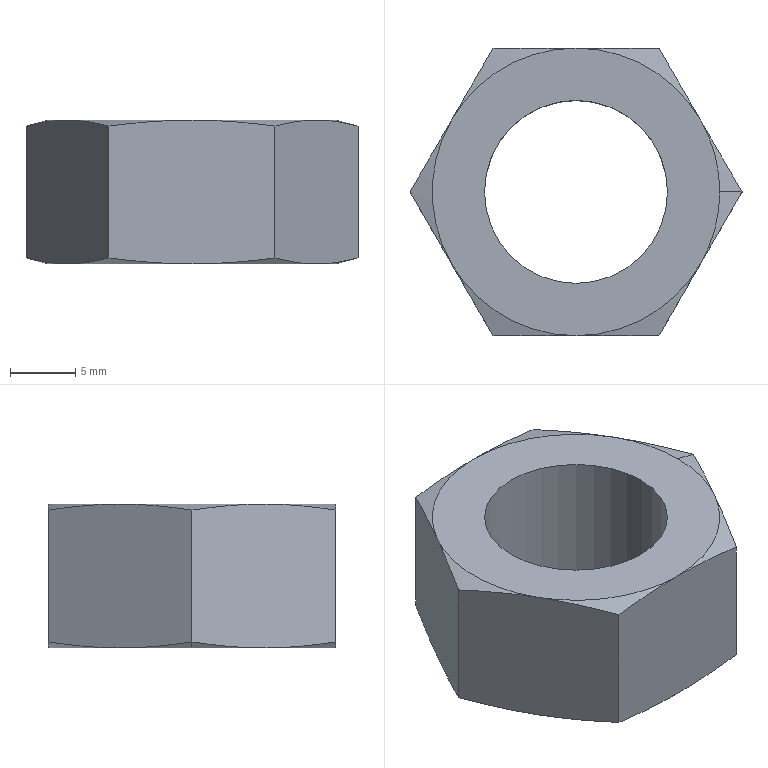Part | SolidWorks | features Cut 2, Chamfer 1, Extrusion 1 | 1 solid | 24 faces | box 25.4 x 21.997 x 11 mm | volume 2905 mm3 | cone 14 | plane 8 | cylinder 2 | commonest cylinder face diameters 14 x2
STEP:
#1=CARTESIAN_POINT('',(10.999,0.,11.));
#2=VERTEX_POINT('',#1);
#3=CARTESIAN_POINT('',(9.525,5.499,11.));
#4=VERTEX_POINT('',#3);
#5=CARTESIAN_POINT('',(0.,0.,11.));
#6=DIRECTION('',(0.,0.,1.));
#7=DIRECTION('',(1.,0.,0.));
#8=AXIS2_PLACEMENT_3D('',#5,#6,#7);
#9=CIRCLE('',#8,10.999);
#10=EDGE_CURVE('',#2,#4,#9,.T.);
#11=ORIENTED_EDGE('',*,*,#10,.F.);
#12=CARTESIAN_POINT('',(12.7,0.,10.544));
#13=VERTEX_POINT('',#12);
#14=CARTESIAN_POINT('',(10.999,0.,11.));
#15=DIRECTION('',(0.9659,0.,-0.2588));
#16=VECTOR('',#15,1000.);
#17=LINE('',#14,#16);
#18=EDGE_CURVE('',#2,#13,#17,.T.);
#19=ORIENTED_EDGE('',*,*,#18,.T.);
#20=CARTESIAN_POINT('',(12.7,0.,10.544));
#21=CARTESIAN_POINT('',(12.171,0.9165,10.686));
#22=CARTESIAN_POINT('',(11.642,1.833,10.801));
#23=CARTESIAN_POINT('',(10.583,3.666,10.958));
#24=CARTESIAN_POINT('',(10.054,4.583,11.));
#25=CARTESIAN_POINT('',(9.525,5.499,11.));
#26=B_SPLINE_CURVE_WITH_KNOTS('',3,(#20,#21,#22,#23,#24,#25),.UNSPECIFIED.,.F.,.F.,(4,2,4),(0.000000231,0.003175,0.00635),.UNSPECIFIED.);
#27=EDGE_CURVE('',#13,#4,#26,.T.);
#28=ORIENTED_EDGE('',*,*,#27,.T.);
#29=EDGE_LOOP('',(#11,#19,#28));
#30=FACE_OUTER_BOUND('',#29,.T.);
#31=CARTESIAN_POINT('',(0.,0.,11.));
#32=DIRECTION('',(0.,0.,-1.));
#33=DIRECTION('',(1.,0.,0.));
#34=AXIS2_PLACEMENT_3D('',#31,#32,#33);
#35=CONICAL_SURFACE('',#34,10.999,1.309);
#36=ADVANCED_FACE('',(#30),#35,.T.);
#37=CARTESIAN_POINT('',(-10.999,0.,0.));
#38=VERTEX_POINT('',#37);
#39=CARTESIAN_POINT('',(-9.525,5.499,0.));
#40=VERTEX_POINT('',#39);
#41=CARTESIAN_POINT('',(0.,0.,0.));
#42=DIRECTION('',(0.,0.,-1.));
#43=DIRECTION('',(-1.,0.,0.));
#44=AXIS2_PLACEMENT_3D('',#41,#42,#43);
#45=CIRCLE('',#44,10.999);
#46=EDGE_CURVE('',#38,#40,#45,.T.);
#47=ORIENTED_EDGE('',*,*,#46,.F.);
#48=CARTESIAN_POINT('',(-12.7,0.,0.4559));
#49=VERTEX_POINT('',#48);
#50=CARTESIAN_POINT('',(-10.999,0.,0.));
#51=DIRECTION('',(-0.9659,0.,0.2588));
#52=VECTOR('',#51,1000.);
#53=LINE('',#50,#52);
#54=EDGE_CURVE('',#38,#49,#53,.T.);
#55=ORIENTED_EDGE('',*,*,#54,.T.);
#56=CARTESIAN_POINT('',(-12.7,0.,0.4559));
#57=CARTESIAN_POINT('',(-12.171,0.9165,0.3141));
#58=CARTESIAN_POINT('',(-11.642,1.833,0.199));
#59=CARTESIAN_POINT('',(-10.583,3.666,0.04169));
#60=CARTESIAN_POINT('',(-10.054,4.583,0.));
#61=CARTESIAN_POINT('',(-9.525,5.499,0.));
#62=B_SPLINE_CURVE_WITH_KNOTS('',3,(#56,#57,#58,#59,#60,#61),.UNSPECIFIED.,.F.,.F.,(4,2,4),(0.000000231,0.003175,0.00635),.UNSPECIFIED.);
#63=EDGE_CURVE('',#49,#40,#62,.T.);
#64=ORIENTED_EDGE('',*,*,#63,.T.);
#65=EDGE_LOOP('',(#47,#55,#64));
#66=FACE_OUTER_BOUND('',#65,.T.);
#67=CARTESIAN_POINT('',(0.,0.,0.));
#68=DIRECTION('',(0.,0.,1.));
#69=DIRECTION('',(-1.,0.,0.));
#70=AXIS2_PLACEMENT_3D('',#67,#68,#69);
#71=CONICAL_SURFACE('',#70,10.999,1.309);
#72=ADVANCED_FACE('',(#66),#71,.T.);
#73=CARTESIAN_POINT('',(-7.,0.,11.));
#74=VERTEX_POINT('',#73);
#75=CARTESIAN_POINT('',(7.,0.,11.));
#76=VERTEX_POINT('',#75);
#77=CARTESIAN_POINT('',(0.,0.,11.));
#78=DIRECTION('',(0.,0.,1.));
#79=DIRECTION('',(1.,0.,0.));
#80=AXIS2_PLACEMENT_3D('',#77,#78,#79);
#81=CIRCLE('',#80,7.);
#82=EDGE_CURVE('',#74,#76,#81,.T.);
#83=ORIENTED_EDGE('',*,*,#82,.T.);
#84=CARTESIAN_POINT('',(7.,0.,0.));
#85=VERTEX_POINT('',#84);
#86=CARTESIAN_POINT('',(7.,0.,11.));
#87=DIRECTION('',(0.,0.,-1.));
#88=VECTOR('',#87,1000.);
#89=LINE('',#86,#88);
#90=EDGE_CURVE('',#76,#85,#89,.T.);
#91=ORIENTED_EDGE('',*,*,#90,.T.);
#92=CARTESIAN_POINT('',(-7.,0.,0.));
#93=VERTEX_POINT('',#92);
#94=CARTESIAN_POINT('',(0.,0.,0.));
#95=DIRECTION('',(0.,0.,1.));
#96=DIRECTION('',(1.,0.,0.));
#97=AXIS2_PLACEMENT_3D('',#94,#95,#96);
#98=CIRCLE('',#97,7.);
#99=EDGE_CURVE('',#93,#85,#98,.T.);
#100=ORIENTED_EDGE('',*,*,#99,.F.);
#101=CARTESIAN_POINT('',(-7.,0.,11.));
#102=DIRECTION('',(0.,0.,-1.));
#103=VECTOR('',#102,1000.);
#104=LINE('',#101,#103);
#105=EDGE_CURVE('',#74,#93,#104,.T.);
#106=ORIENTED_EDGE('',*,*,#105,.F.);
#107=EDGE_LOOP('',(#83,#91,#100,#106));
#108=FACE_OUTER_BOUND('',#107,.T.);
#109=CARTESIAN_POINT('',(0.,0.,11.));
#110=DIRECTION('',(0.,0.,-1.));
#111=DIRECTION('',(-1.,0.,0.));
#112=AXIS2_PLACEMENT_3D('',#109,#110,#111);
#113=CYLINDRICAL_SURFACE('',#112,7.);
#114=ADVANCED_FACE('',(#108),#113,.F.);
#115=ORIENTED_EDGE('',*,*,#27,.F.);
#116=CARTESIAN_POINT('',(12.7,0.,0.4559));
#117=VERTEX_POINT('',#116);
#118=CARTESIAN_POINT('',(12.7,0.,11.));
#119=DIRECTION('',(0.,0.,-1.));
#120=VECTOR('',#119,1000.);
#121=LINE('',#118,#120);
#122=EDGE_CURVE('',#13,#117,#121,.T.);
#123=ORIENTED_EDGE('',*,*,#122,.T.);
#124=CARTESIAN_POINT('',(9.525,5.499,0.));
#125=VERTEX_POINT('',#124);
#126=CARTESIAN_POINT('',(9.525,5.499,0.));
#127=CARTESIAN_POINT('',(10.054,4.583,0.));
#128=CARTESIAN_POINT('',(10.583,3.666,0.04169));
#129=CARTESIAN_POINT('',(11.642,1.833,0.199));
#130=CARTESIAN_POINT('',(12.171,0.9165,0.3141));
#131=CARTESIAN_POINT('',(12.7,0.,0.4559));
#132=B_SPLINE_CURVE_WITH_KNOTS('',3,(#126,#127,#128,#129,#130,#131),.UNSPECIFIED.,.F.,.F.,(4,2,4),(0.00635,0.009525,0.0127),.UNSPECIFIED.);
#133=EDGE_CURVE('',#125,#117,#132,.T.);
#134=ORIENTED_EDGE('',*,*,#133,.F.);
#135=CARTESIAN_POINT('',(6.35,10.999,0.4559));
#136=VERTEX_POINT('',#135);
#137=CARTESIAN_POINT('',(6.35,10.999,0.4559));
#138=CARTESIAN_POINT('',(6.879,10.082,0.3141));
#139=CARTESIAN_POINT('',(7.408,9.165,0.199));
#140=CARTESIAN_POINT('',(8.467,7.332,0.04169));
#141=CARTESIAN_POINT('',(8.996,6.416,0.));
#142=CARTESIAN_POINT('',(9.525,5.499,0.));
#143=B_SPLINE_CURVE_WITH_KNOTS('',3,(#137,#138,#139,#140,#141,#142),.UNSPECIFIED.,.F.,.F.,(4,2,4),(0.000000231,0.003175,0.00635),.UNSPECIFIED.);
#144=EDGE_CURVE('',#136,#125,#143,.T.);
#145=ORIENTED_EDGE('',*,*,#144,.F.);
#146=CARTESIAN_POINT('',(6.35,10.999,10.544));
#147=VERTEX_POINT('',#146);
#148=CARTESIAN_POINT('',(6.35,10.999,11.));
#149=DIRECTION('',(0.,0.,-1.));
#150=VECTOR('',#149,1000.);
#151=LINE('',#148,#150);
#152=EDGE_CURVE('',#147,#136,#151,.T.);
#153=ORIENTED_EDGE('',*,*,#152,.F.);
#154=CARTESIAN_POINT('',(9.525,5.499,11.));
#155=CARTESIAN_POINT('',(8.996,6.416,11.));
#156=CARTESIAN_POINT('',(8.467,7.332,10.958));
#157=CARTESIAN_POINT('',(7.408,9.165,10.801));
#158=CARTESIAN_POINT('',(6.879,10.082,10.686));
#159=CARTESIAN_POINT('',(6.35,10.999,10.544));
#160=B_SPLINE_CURVE_WITH_KNOTS('',3,(#154,#155,#156,#157,#158,#159),.UNSPECIFIED.,.F.,.F.,(4,2,4),(0.00635,0.009525,0.0127),.UNSPECIFIED.);
#161=EDGE_CURVE('',#4,#147,#160,.T.);
#162=ORIENTED_EDGE('',*,*,#161,.F.);
#163=EDGE_LOOP('',(#115,#123,#134,#145,#153,#162));
#164=FACE_OUTER_BOUND('',#163,.T.);
#165=CARTESIAN_POINT('',(12.7,0.,11.));
#166=DIRECTION('',(-0.866,-0.5,0.));
#167=DIRECTION('',(0.5,-0.866,0.));
#168=AXIS2_PLACEMENT_3D('',#165,#166,#167);
#169=PLANE('',#168);
#170=ADVANCED_FACE('',(#164),#169,.F.);
#171=CARTESIAN_POINT('',(0.,10.999,11.));
#172=VERTEX_POINT('',#171);
#173=CARTESIAN_POINT('',(6.35,10.999,10.544));
#174=CARTESIAN_POINT('',(5.293,10.999,10.686));
#175=CARTESIAN_POINT('',(4.236,10.999,10.801));
#176=CARTESIAN_POINT('',(2.12,10.999,10.958));
#177=CARTESIAN_POINT('',(1.06,10.999,11.));
#178=CARTESIAN_POINT('',(0.,10.999,11.));
#179=B_SPLINE_CURVE_WITH_KNOTS('',3,(#173,#174,#175,#176,#177,#178),.UNSPECIFIED.,.F.,.F.,(4,2,4),(0.03237,0.03557,0.03876),.UNSPECIFIED.);
#180=EDGE_CURVE('',#147,#172,#179,.T.);
#181=ORIENTED_EDGE('',*,*,#180,.F.);
#182=ORIENTED_EDGE('',*,*,#152,.T.);
#183=CARTESIAN_POINT('',(0.,10.999,0.));
#184=VERTEX_POINT('',#183);
#185=CARTESIAN_POINT('',(0.,10.999,0.));
#186=CARTESIAN_POINT('',(1.06,10.999,0.));
#187=CARTESIAN_POINT('',(2.12,10.999,0.04184));
#188=CARTESIAN_POINT('',(4.236,10.999,0.1993));
#189=CARTESIAN_POINT('',(5.293,10.999,0.3144));
#190=CARTESIAN_POINT('',(6.35,10.999,0.4559));
#191=B_SPLINE_CURVE_WITH_KNOTS('',3,(#185,#186,#187,#188,#189,#190),.UNSPECIFIED.,.F.,.F.,(4,2,4),(0.01717,0.02038,0.02358),.UNSPECIFIED.);
#192=EDGE_CURVE('',#184,#136,#191,.T.);
#193=ORIENTED_EDGE('',*,*,#192,.F.);
#194=CARTESIAN_POINT('',(-6.35,10.999,0.4559));
#195=VERTEX_POINT('',#194);
#196=CARTESIAN_POINT('',(-6.35,10.999,0.4559));
#197=CARTESIAN_POINT('',(-5.295,10.999,0.3145));
#198=CARTESIAN_POINT('',(-4.233,10.999,0.1989));
#199=CARTESIAN_POINT('',(-2.115,10.999,0.04158));
#200=CARTESIAN_POINT('',(-1.057,10.999,0.));
#201=CARTESIAN_POINT('',(0.,10.999,0.));
#202=B_SPLINE_CURVE_WITH_KNOTS('',3,(#196,#197,#198,#199,#200,#201),.UNSPECIFIED.,.F.,.F.,(4,2,4),(0.01079,0.01398,0.01717),.UNSPECIFIED.);
#203=EDGE_CURVE('',#195,#184,#202,.T.);
#204=ORIENTED_EDGE('',*,*,#203,.F.);
#205=CARTESIAN_POINT('',(-6.35,10.999,10.544));
#206=VERTEX_POINT('',#205);
#207=CARTESIAN_POINT('',(-6.35,10.999,11.));
#208=DIRECTION('',(0.,0.,-1.));
#209=VECTOR('',#208,1000.);
#210=LINE('',#207,#209);
#211=EDGE_CURVE('',#206,#195,#210,.T.);
#212=ORIENTED_EDGE('',*,*,#211,.F.);
#213=CARTESIAN_POINT('',(0.,10.999,11.));
#214=CARTESIAN_POINT('',(-1.057,10.999,11.));
#215=CARTESIAN_POINT('',(-2.115,10.999,10.958));
#216=CARTESIAN_POINT('',(-4.233,10.999,10.801));
#217=CARTESIAN_POINT('',(-5.295,10.999,10.685));
#218=CARTESIAN_POINT('',(-6.35,10.999,10.544));
#219=B_SPLINE_CURVE_WITH_KNOTS('',3,(#213,#214,#215,#216,#217,#218),.UNSPECIFIED.,.F.,.F.,(4,2,4),(0.03876,0.04194,0.04513),.UNSPECIFIED.);
#220=EDGE_CURVE('',#172,#206,#219,.T.);
#221=ORIENTED_EDGE('',*,*,#220,.F.);
#222=EDGE_LOOP('',(#181,#182,#193,#204,#212,#221));
#223=FACE_OUTER_BOUND('',#222,.T.);
#224=CARTESIAN_POINT('',(6.35,10.999,11.));
#225=DIRECTION('',(0.,-1.,0.));
#226=DIRECTION('',(1.,0.,0.));
#227=AXIS2_PLACEMENT_3D('',#224,#225,#226);
#228=PLANE('',#227);
#229=ADVANCED_FACE('',(#223),#228,.F.);
#230=CARTESIAN_POINT('',(-9.525,5.499,11.));
#231=VERTEX_POINT('',#230);
#232=CARTESIAN_POINT('',(-6.35,10.999,10.544));
#233=CARTESIAN_POINT('',(-6.879,10.082,10.686));
#234=CARTESIAN_POINT('',(-7.408,9.165,10.801));
#235=CARTESIAN_POINT('',(-8.467,7.332,10.958));
#236=CARTESIAN_POINT('',(-8.996,6.416,11.));
#237=CARTESIAN_POINT('',(-9.525,5.499,11.));
#238=B_SPLINE_CURVE_WITH_KNOTS('',3,(#232,#233,#234,#235,#236,#237),.UNSPECIFIED.,.F.,.F.,(4,2,4),(0.000000231,0.003175,0.00635),.UNSPECIFIED.);
#239=EDGE_CURVE('',#206,#231,#238,.T.);
#240=ORIENTED_EDGE('',*,*,#239,.F.);
#241=ORIENTED_EDGE('',*,*,#211,.T.);
#242=CARTESIAN_POINT('',(-9.525,5.499,0.));
#243=CARTESIAN_POINT('',(-8.996,6.416,0.));
#244=CARTESIAN_POINT('',(-8.467,7.332,0.04169));
#245=CARTESIAN_POINT('',(-7.408,9.165,0.199));
#246=CARTESIAN_POINT('',(-6.879,10.082,0.3141));
#247=CARTESIAN_POINT('',(-6.35,10.999,0.4559));
#248=B_SPLINE_CURVE_WITH_KNOTS('',3,(#242,#243,#244,#245,#246,#247),.UNSPECIFIED.,.F.,.F.,(4,2,4),(0.00635,0.009525,0.0127),.UNSPECIFIED.);
#249=EDGE_CURVE('',#40,#195,#248,.T.);
#250=ORIENTED_EDGE('',*,*,#249,.F.);
#251=ORIENTED_EDGE('',*,*,#63,.F.);
#252=CARTESIAN_POINT('',(-12.7,0.,10.544));
#253=VERTEX_POINT('',#252);
#254=CARTESIAN_POINT('',(-12.7,0.,11.));
#255=DIRECTION('',(0.,0.,-1.));
#256=VECTOR('',#255,1000.);
#257=LINE('',#254,#256);
#258=EDGE_CURVE('',#253,#49,#257,.T.);
#259=ORIENTED_EDGE('',*,*,#258,.F.);
#260=CARTESIAN_POINT('',(-9.525,5.499,11.));
#261=CARTESIAN_POINT('',(-10.054,4.583,11.));
#262=CARTESIAN_POINT('',(-10.583,3.666,10.958));
#263=CARTESIAN_POINT('',(-11.642,1.833,10.801));
#264=CARTESIAN_POINT('',(-12.171,0.9165,10.686));
#265=CARTESIAN_POINT('',(-12.7,0.,10.544));
#266=B_SPLINE_CURVE_WITH_KNOTS('',3,(#260,#261,#262,#263,#264,#265),.UNSPECIFIED.,.F.,.F.,(4,2,4),(0.00635,0.009525,0.0127),.UNSPECIFIED.);
#267=EDGE_CURVE('',#231,#253,#266,.T.);
#268=ORIENTED_EDGE('',*,*,#267,.F.);
#269=EDGE_LOOP('',(#240,#241,#250,#251,#259,#268));
#270=FACE_OUTER_BOUND('',#269,.T.);
#271=CARTESIAN_POINT('',(-6.35,10.999,11.));
#272=DIRECTION('',(0.866,-0.5,0.));
#273=DIRECTION('',(0.5,0.866,0.));
#274=AXIS2_PLACEMENT_3D('',#271,#272,#273);
#275=PLANE('',#274);
#276=ADVANCED_FACE('',(#270),#275,.F.);
#277=CARTESIAN_POINT('',(-9.525,-5.499,11.));
#278=VERTEX_POINT('',#277);
#279=CARTESIAN_POINT('',(-12.7,0.,10.544));
#280=CARTESIAN_POINT('',(-12.171,-0.9165,10.686));
#281=CARTESIAN_POINT('',(-11.642,-1.833,10.801));
#282=CARTESIAN_POINT('',(-10.583,-3.666,10.958));
#283=CARTESIAN_POINT('',(-10.054,-4.583,11.));
#284=CARTESIAN_POINT('',(-9.525,-5.499,11.));
#285=B_SPLINE_CURVE_WITH_KNOTS('',3,(#279,#280,#281,#282,#283,#284),.UNSPECIFIED.,.F.,.F.,(4,2,4),(0.000000231,0.003175,0.00635),.UNSPECIFIED.);
#286=EDGE_CURVE('',#253,#278,#285,.T.);
#287=ORIENTED_EDGE('',*,*,#286,.F.);
#288=ORIENTED_EDGE('',*,*,#258,.T.);
#289=CARTESIAN_POINT('',(-9.525,-5.499,0.));
#290=VERTEX_POINT('',#289);
#291=CARTESIAN_POINT('',(-9.525,-5.499,0.));
#292=CARTESIAN_POINT('',(-10.054,-4.583,0.));
#293=CARTESIAN_POINT('',(-10.583,-3.666,0.04169));
#294=CARTESIAN_POINT('',(-11.642,-1.833,0.199));
#295=CARTESIAN_POINT('',(-12.171,-0.9165,0.3141));
#296=CARTESIAN_POINT('',(-12.7,0.,0.4559));
#297=B_SPLINE_CURVE_WITH_KNOTS('',3,(#291,#292,#293,#294,#295,#296),.UNSPECIFIED.,.F.,.F.,(4,2,4),(0.00635,0.009525,0.0127),.UNSPECIFIED.);
#298=EDGE_CURVE('',#290,#49,#297,.T.);
#299=ORIENTED_EDGE('',*,*,#298,.F.);
#300=CARTESIAN_POINT('',(-6.35,-10.999,0.4559));
#301=VERTEX_POINT('',#300);
#302=CARTESIAN_POINT('',(-6.35,-10.999,0.4559));
#303=CARTESIAN_POINT('',(-6.879,-10.082,0.3141));
#304=CARTESIAN_POINT('',(-7.408,-9.165,0.199));
#305=CARTESIAN_POINT('',(-8.467,-7.332,0.04169));
#306=CARTESIAN_POINT('',(-8.996,-6.416,0.));
#307=CARTESIAN_POINT('',(-9.525,-5.499,0.));
#308=B_SPLINE_CURVE_WITH_KNOTS('',3,(#302,#303,#304,#305,#306,#307),.UNSPECIFIED.,.F.,.F.,(4,2,4),(0.000000231,0.003175,0.00635),.UNSPECIFIED.);
#309=EDGE_CURVE('',#301,#290,#308,.T.);
#310=ORIENTED_EDGE('',*,*,#309,.F.);
#311=CARTESIAN_POINT('',(-6.35,-10.999,10.544));
#312=VERTEX_POINT('',#311);
#313=CARTESIAN_POINT('',(-6.35,-10.999,11.));
#314=DIRECTION('',(0.,0.,-1.));
#315=VECTOR('',#314,1000.);
#316=LINE('',#313,#315);
#317=EDGE_CURVE('',#312,#301,#316,.T.);
#318=ORIENTED_EDGE('',*,*,#317,.F.);
#319=CARTESIAN_POINT('',(-9.525,-5.499,11.));
#320=CARTESIAN_POINT('',(-8.996,-6.416,11.));
#321=CARTESIAN_POINT('',(-8.467,-7.332,10.958));
#322=CARTESIAN_POINT('',(-7.408,-9.165,10.801));
#323=CARTESIAN_POINT('',(-6.879,-10.082,10.686));
#324=CARTESIAN_POINT('',(-6.35,-10.999,10.544));
#325=B_SPLINE_CURVE_WITH_KNOTS('',3,(#319,#320,#321,#322,#323,#324),.UNSPECIFIED.,.F.,.F.,(4,2,4),(0.00635,0.009525,0.0127),.UNSPECIFIED.);
#326=EDGE_CURVE('',#278,#312,#325,.T.);
#327=ORIENTED_EDGE('',*,*,#326,.F.);
#328=EDGE_LOOP('',(#287,#288,#299,#310,#318,#327));
#329=FACE_OUTER_BOUND('',#328,.T.);
#330=CARTESIAN_POINT('',(-12.7,0.,11.));
#331=DIRECTION('',(0.866,0.5,0.));
#332=DIRECTION('',(-0.5,0.866,0.));
#333=AXIS2_PLACEMENT_3D('',#330,#331,#332);
#334=PLANE('',#333);
#335=ADVANCED_FACE('',(#329),#334,.F.);
#336=CARTESIAN_POINT('',(0.,-10.999,11.));
#337=VERTEX_POINT('',#336);
#338=CARTESIAN_POINT('',(-6.35,-10.999,10.544));
#339=CARTESIAN_POINT('',(-5.295,-10.999,10.685));
#340=CARTESIAN_POINT('',(-4.233,-10.999,10.801));
#341=CARTESIAN_POINT('',(-2.115,-10.999,10.958));
#342=CARTESIAN_POINT('',(-1.057,-10.999,11.));
#343=CARTESIAN_POINT('',(0.,-10.999,11.));
#344=B_SPLINE_CURVE_WITH_KNOTS('',3,(#338,#339,#340,#341,#342,#343),.UNSPECIFIED.,.F.,.F.,(4,2,4),(0.01079,0.01398,0.01717),.UNSPECIFIED.);
#345=EDGE_CURVE('',#312,#337,#344,.T.);
#346=ORIENTED_EDGE('',*,*,#345,.F.);
#347=ORIENTED_EDGE('',*,*,#317,.T.);
#348=CARTESIAN_POINT('',(0.,-10.999,0.));
#349=VERTEX_POINT('',#348);
#350=CARTESIAN_POINT('',(0.,-10.999,0.));
#351=CARTESIAN_POINT('',(-1.057,-10.999,0.));
#352=CARTESIAN_POINT('',(-2.115,-10.999,0.04158));
#353=CARTESIAN_POINT('',(-4.233,-10.999,0.1989));
#354=CARTESIAN_POINT('',(-5.295,-10.999,0.3145));
#355=CARTESIAN_POINT('',(-6.35,-10.999,0.4559));
#356=B_SPLINE_CURVE_WITH_KNOTS('',3,(#350,#351,#352,#353,#354,#355),.UNSPECIFIED.,.F.,.F.,(4,2,4),(0.03876,0.04194,0.04513),.UNSPECIFIED.);
#357=EDGE_CURVE('',#349,#301,#356,.T.);
#358=ORIENTED_EDGE('',*,*,#357,.F.);
#359=CARTESIAN_POINT('',(6.35,-10.999,0.4559));
#360=VERTEX_POINT('',#359);
#361=CARTESIAN_POINT('',(6.35,-10.999,0.4559));
#362=CARTESIAN_POINT('',(5.293,-10.999,0.3144));
#363=CARTESIAN_POINT('',(4.236,-10.999,0.1993));
#364=CARTESIAN_POINT('',(2.12,-10.999,0.04184));
#365=CARTESIAN_POINT('',(1.06,-10.999,0.));
#366=CARTESIAN_POINT('',(0.,-10.999,0.));
#367=B_SPLINE_CURVE_WITH_KNOTS('',3,(#361,#362,#363,#364,#365,#366),.UNSPECIFIED.,.F.,.F.,(4,2,4),(0.03237,0.03557,0.03876),.UNSPECIFIED.);
#368=EDGE_CURVE('',#360,#349,#367,.T.);
#369=ORIENTED_EDGE('',*,*,#368,.F.);
#370=CARTESIAN_POINT('',(6.35,-10.999,10.544));
#371=VERTEX_POINT('',#370);
#372=CARTESIAN_POINT('',(6.35,-10.999,11.));
#373=DIRECTION('',(0.,0.,-1.));
#374=VECTOR('',#373,1000.);
#375=LINE('',#372,#374);
#376=EDGE_CURVE('',#371,#360,#375,.T.);
#377=ORIENTED_EDGE('',*,*,#376,.F.);
#378=CARTESIAN_POINT('',(0.,-10.999,11.));
#379=CARTESIAN_POINT('',(1.06,-10.999,11.));
#380=CARTESIAN_POINT('',(2.12,-10.999,10.958));
#381=CARTESIAN_POINT('',(4.236,-10.999,10.801));
#382=CARTESIAN_POINT('',(5.293,-10.999,10.686));
#383=CARTESIAN_POINT('',(6.35,-10.999,10.544));
#384=B_SPLINE_CURVE_WITH_KNOTS('',3,(#378,#379,#380,#381,#382,#383),.UNSPECIFIED.,.F.,.F.,(4,2,4),(0.01717,0.02038,0.02358),.UNSPECIFIED.);
#385=EDGE_CURVE('',#337,#371,#384,.T.);
#386=ORIENTED_EDGE('',*,*,#385,.F.);
#387=EDGE_LOOP('',(#346,#347,#358,#369,#377,#386));
#388=FACE_OUTER_BOUND('',#387,.T.);
#389=CARTESIAN_POINT('',(-6.35,-10.999,11.));
#390=DIRECTION('',(0.,1.,0.));
#391=DIRECTION('',(-1.,0.,0.));
#392=AXIS2_PLACEMENT_3D('',#389,#390,#391);
#393=PLANE('',#392);
#394=ADVANCED_FACE('',(#388),#393,.F.);
#395=CARTESIAN_POINT('',(9.525,-5.499,11.));
#396=VERTEX_POINT('',#395);
#397=CARTESIAN_POINT('',(6.35,-10.999,10.544));
#398=CARTESIAN_POINT('',(6.879,-10.082,10.686));
#399=CARTESIAN_POINT('',(7.408,-9.165,10.801));
#400=CARTESIAN_POINT('',(8.467,-7.332,10.958));
#401=CARTESIAN_POINT('',(8.996,-6.416,11.));
#402=CARTESIAN_POINT('',(9.525,-5.499,11.));
#403=B_SPLINE_CURVE_WITH_KNOTS('',3,(#397,#398,#399,#400,#401,#402),.UNSPECIFIED.,.F.,.F.,(4,2,4),(0.000000231,0.003175,0.00635),.UNSPECIFIED.);
#404=EDGE_CURVE('',#371,#396,#403,.T.);
#405=ORIENTED_EDGE('',*,*,#404,.F.);
#406=ORIENTED_EDGE('',*,*,#376,.T.);
#407=CARTESIAN_POINT('',(9.525,-5.499,0.));
#408=VERTEX_POINT('',#407);
#409=CARTESIAN_POINT('',(9.525,-5.499,0.));
#410=CARTESIAN_POINT('',(8.996,-6.416,0.));
#411=CARTESIAN_POINT('',(8.467,-7.332,0.04169));
#412=CARTESIAN_POINT('',(7.408,-9.165,0.199));
#413=CARTESIAN_POINT('',(6.879,-10.082,0.3141));
#414=CARTESIAN_POINT('',(6.35,-10.999,0.4559));
#415=B_SPLINE_CURVE_WITH_KNOTS('',3,(#409,#410,#411,#412,#413,#414),.UNSPECIFIED.,.F.,.F.,(4,2,4),(0.00635,0.009525,0.0127),.UNSPECIFIED.);
#416=EDGE_CURVE('',#408,#360,#415,.T.);
#417=ORIENTED_EDGE('',*,*,#416,.F.);
#418=CARTESIAN_POINT('',(12.7,0.,0.4559));
#419=CARTESIAN_POINT('',(12.171,-0.9165,0.3141));
#420=CARTESIAN_POINT('',(11.642,-1.833,0.199));
#421=CARTESIAN_POINT('',(10.583,-3.666,0.04169));
#422=CARTESIAN_POINT('',(10.054,-4.583,0.));
#423=CARTESIAN_POINT('',(9.525,-5.499,0.));
#424=B_SPLINE_CURVE_WITH_KNOTS('',3,(#418,#419,#420,#421,#422,#423),.UNSPECIFIED.,.F.,.F.,(4,2,4),(0.000000231,0.003175,0.00635),.UNSPECIFIED.);
#425=EDGE_CURVE('',#117,#408,#424,.T.);
#426=ORIENTED_EDGE('',*,*,#425,.F.);
#427=ORIENTED_EDGE('',*,*,#122,.F.);
#428=CARTESIAN_POINT('',(9.525,-5.499,11.));
#429=CARTESIAN_POINT('',(10.054,-4.583,11.));
#430=CARTESIAN_POINT('',(10.583,-3.666,10.958));
#431=CARTESIAN_POINT('',(11.642,-1.833,10.801));
#432=CARTESIAN_POINT('',(12.171,-0.9165,10.686));
#433=CARTESIAN_POINT('',(12.7,0.,10.544));
#434=B_SPLINE_CURVE_WITH_KNOTS('',3,(#428,#429,#430,#431,#432,#433),.UNSPECIFIED.,.F.,.F.,(4,2,4),(0.00635,0.009525,0.0127),.UNSPECIFIED.);
#435=EDGE_CURVE('',#396,#13,#434,.T.);
#436=ORIENTED_EDGE('',*,*,#435,.F.);
#437=EDGE_LOOP('',(#405,#406,#417,#426,#427,#436));
#438=FACE_OUTER_BOUND('',#437,.T.);
#439=CARTESIAN_POINT('',(6.35,-10.999,11.));
#440=DIRECTION('',(-0.866,0.5,0.));
#441=DIRECTION('',(-0.5,-0.866,0.));
#442=AXIS2_PLACEMENT_3D('',#439,#440,#441);
#443=PLANE('',#442);
#444=ADVANCED_FACE('',(#438),#443,.F.);
#445=ORIENTED_EDGE('',*,*,#82,.F.);
#446=CARTESIAN_POINT('',(0.,0.,11.));
#447=DIRECTION('',(0.,0.,1.));
#448=DIRECTION('',(1.,0.,0.));
#449=AXIS2_PLACEMENT_3D('',#446,#447,#448);
#450=CIRCLE('',#449,7.);
#451=EDGE_CURVE('',#76,#74,#450,.T.);
#452=ORIENTED_EDGE('',*,*,#451,.F.);
#453=EDGE_LOOP('',(#445,#452));
#454=FACE_BOUND('',#453,.T.);
#455=CARTESIAN_POINT('',(0.,0.,11.));
#456=DIRECTION('',(0.,0.,1.));
#457=DIRECTION('',(1.,0.,0.));
#458=AXIS2_PLACEMENT_3D('',#455,#456,#457);
#459=CIRCLE('',#458,10.999);
#460=EDGE_CURVE('',#396,#2,#459,.T.);
#461=ORIENTED_EDGE('',*,*,#460,.T.);
#462=ORIENTED_EDGE('',*,*,#10,.T.);
#463=CARTESIAN_POINT('',(0.,0.,11.));
#464=DIRECTION('',(0.,0.,1.));
#465=DIRECTION('',(1.,0.,0.));
#466=AXIS2_PLACEMENT_3D('',#463,#464,#465);
#467=CIRCLE('',#466,10.999);
#468=EDGE_CURVE('',#4,#172,#467,.T.);
#469=ORIENTED_EDGE('',*,*,#468,.T.);
#470=CARTESIAN_POINT('',(0.,0.,11.));
#471=DIRECTION('',(0.,0.,1.));
#472=DIRECTION('',(1.,0.,0.));
#473=AXIS2_PLACEMENT_3D('',#470,#471,#472);
#474=CIRCLE('',#473,10.999);
#475=EDGE_CURVE('',#172,#231,#474,.T.);
#476=ORIENTED_EDGE('',*,*,#475,.T.);
#477=CARTESIAN_POINT('',(0.,0.,11.));
#478=DIRECTION('',(0.,0.,1.));
#479=DIRECTION('',(1.,0.,0.));
#480=AXIS2_PLACEMENT_3D('',#477,#478,#479);
#481=CIRCLE('',#480,10.999);
#482=EDGE_CURVE('',#231,#278,#481,.T.);
#483=ORIENTED_EDGE('',*,*,#482,.T.);
#484=CARTESIAN_POINT('',(0.,0.,11.));
#485=DIRECTION('',(0.,0.,1.));
#486=DIRECTION('',(1.,0.,0.));
#487=AXIS2_PLACEMENT_3D('',#484,#485,#486);
#488=CIRCLE('',#487,10.999);
#489=EDGE_CURVE('',#278,#337,#488,.T.);
#490=ORIENTED_EDGE('',*,*,#489,.T.);
#491=CARTESIAN_POINT('',(0.,0.,11.));
#492=DIRECTION('',(0.,0.,1.));
#493=DIRECTION('',(1.,0.,0.));
#494=AXIS2_PLACEMENT_3D('',#491,#492,#493);
#495=CIRCLE('',#494,10.999);
#496=EDGE_CURVE('',#337,#396,#495,.T.);
#497=ORIENTED_EDGE('',*,*,#496,.T.);
#498=EDGE_LOOP('',(#461,#462,#469,#476,#483,#490,#497));
#499=FACE_OUTER_BOUND('',#498,.T.);
#500=CARTESIAN_POINT('',(6.35,10.999,11.));
#501=DIRECTION('',(0.,0.,1.));
#502=DIRECTION('',(1.,0.,0.));
#503=AXIS2_PLACEMENT_3D('',#500,#501,#502);
#504=PLANE('',#503);
#505=ADVANCED_FACE('',(#454,#499),#504,.T.);
#506=ORIENTED_EDGE('',*,*,#99,.T.);
#507=CARTESIAN_POINT('',(0.,0.,0.));
#508=DIRECTION('',(0.,0.,1.));
#509=DIRECTION('',(1.,0.,0.));
#510=AXIS2_PLACEMENT_3D('',#507,#508,#509);
#511=CIRCLE('',#510,7.);
#512=EDGE_CURVE('',#85,#93,#511,.T.);
#513=ORIENTED_EDGE('',*,*,#512,.T.);
#514=EDGE_LOOP('',(#506,#513));
#515=FACE_BOUND('',#514,.T.);
#516=CARTESIAN_POINT('',(0.,0.,0.));
#517=DIRECTION('',(0.,0.,-1.));
#518=DIRECTION('',(-1.,0.,0.));
#519=AXIS2_PLACEMENT_3D('',#516,#517,#518);
#520=CIRCLE('',#519,10.999);
#521=EDGE_CURVE('',#184,#125,#520,.T.);
#522=ORIENTED_EDGE('',*,*,#521,.T.);
#523=CARTESIAN_POINT('',(0.,0.,0.));
#524=DIRECTION('',(0.,0.,-1.));
#525=DIRECTION('',(-1.,0.,0.));
#526=AXIS2_PLACEMENT_3D('',#523,#524,#525);
#527=CIRCLE('',#526,10.999);
#528=EDGE_CURVE('',#125,#408,#527,.T.);
#529=ORIENTED_EDGE('',*,*,#528,.T.);
#530=CARTESIAN_POINT('',(0.,0.,0.));
#531=DIRECTION('',(0.,0.,-1.));
#532=DIRECTION('',(-1.,0.,0.));
#533=AXIS2_PLACEMENT_3D('',#530,#531,#532);
#534=CIRCLE('',#533,10.999);
#535=EDGE_CURVE('',#408,#349,#534,.T.);
#536=ORIENTED_EDGE('',*,*,#535,.T.);
#537=CARTESIAN_POINT('',(0.,0.,0.));
#538=DIRECTION('',(0.,0.,-1.));
#539=DIRECTION('',(-1.,0.,0.));
#540=AXIS2_PLACEMENT_3D('',#537,#538,#539);
#541=CIRCLE('',#540,10.999);
#542=EDGE_CURVE('',#349,#290,#541,.T.);
#543=ORIENTED_EDGE('',*,*,#542,.T.);
#544=CARTESIAN_POINT('',(0.,0.,0.));
#545=DIRECTION('',(0.,0.,-1.));
#546=DIRECTION('',(-1.,0.,0.));
#547=AXIS2_PLACEMENT_3D('',#544,#545,#546);
#548=CIRCLE('',#547,10.999);
#549=EDGE_CURVE('',#290,#38,#548,.T.);
#550=ORIENTED_EDGE('',*,*,#549,.T.);
#551=ORIENTED_EDGE('',*,*,#46,.T.);
#552=CARTESIAN_POINT('',(0.,0.,0.));
#553=DIRECTION('',(0.,0.,-1.));
#554=DIRECTION('',(-1.,0.,0.));
#555=AXIS2_PLACEMENT_3D('',#552,#553,#554);
#556=CIRCLE('',#555,10.999);
#557=EDGE_CURVE('',#40,#184,#556,.T.);
#558=ORIENTED_EDGE('',*,*,#557,.T.);
#559=EDGE_LOOP('',(#522,#529,#536,#543,#550,#551,#558));
#560=FACE_OUTER_BOUND('',#559,.T.);
#561=CARTESIAN_POINT('',(6.35,10.999,0.));
#562=DIRECTION('',(0.,0.,1.));
#563=DIRECTION('',(1.,0.,0.));
#564=AXIS2_PLACEMENT_3D('',#561,#562,#563);
#565=PLANE('',#564);
#566=ADVANCED_FACE('',(#515,#560),#565,.F.);
#567=ORIENTED_EDGE('',*,*,#90,.F.);
#568=ORIENTED_EDGE('',*,*,#451,.T.);
#569=ORIENTED_EDGE('',*,*,#105,.T.);
#570=ORIENTED_EDGE('',*,*,#512,.F.);
#571=EDGE_LOOP('',(#567,#568,#569,#570));
#572=FACE_OUTER_BOUND('',#571,.T.);
#573=CARTESIAN_POINT('',(0.,0.,11.));
#574=DIRECTION('',(0.,0.,-1.));
#575=DIRECTION('',(-1.,0.,0.));
#576=AXIS2_PLACEMENT_3D('',#573,#574,#575);
#577=CYLINDRICAL_SURFACE('',#576,7.);
#578=ADVANCED_FACE('',(#572),#577,.F.);
#579=ORIENTED_EDGE('',*,*,#368,.T.);
#580=ORIENTED_EDGE('',*,*,#535,.F.);
#581=ORIENTED_EDGE('',*,*,#416,.T.);
#582=EDGE_LOOP('',(#579,#580,#581));
#583=FACE_OUTER_BOUND('',#582,.T.);
#584=CARTESIAN_POINT('',(0.,0.,0.));
#585=DIRECTION('',(0.,0.,1.));
#586=DIRECTION('',(-1.,0.,0.));
#587=AXIS2_PLACEMENT_3D('',#584,#585,#586);
#588=CONICAL_SURFACE('',#587,10.999,1.309);
#589=ADVANCED_FACE('',(#583),#588,.T.);
#590=ORIENTED_EDGE('',*,*,#133,.T.);
#591=ORIENTED_EDGE('',*,*,#425,.T.);
#592=ORIENTED_EDGE('',*,*,#528,.F.);
#593=EDGE_LOOP('',(#590,#591,#592));
#594=FACE_OUTER_BOUND('',#593,.T.);
#595=CARTESIAN_POINT('',(0.,0.,0.));
#596=DIRECTION('',(0.,0.,1.));
#597=DIRECTION('',(-1.,0.,0.));
#598=AXIS2_PLACEMENT_3D('',#595,#596,#597);
#599=CONICAL_SURFACE('',#598,10.999,1.309);
#600=ADVANCED_FACE('',(#594),#599,.T.);
#601=ORIENTED_EDGE('',*,*,#309,.T.);
#602=ORIENTED_EDGE('',*,*,#542,.F.);
#603=ORIENTED_EDGE('',*,*,#357,.T.);
#604=EDGE_LOOP('',(#601,#602,#603));
#605=FACE_OUTER_BOUND('',#604,.T.);
#606=CARTESIAN_POINT('',(0.,0.,0.));
#607=DIRECTION('',(0.,0.,1.));
#608=DIRECTION('',(-1.,0.,0.));
#609=AXIS2_PLACEMENT_3D('',#606,#607,#608);
#610=CONICAL_SURFACE('',#609,10.999,1.309);
#611=ADVANCED_FACE('',(#605),#610,.T.);
#612=ORIENTED_EDGE('',*,*,#54,.F.);
#613=ORIENTED_EDGE('',*,*,#549,.F.);
#614=ORIENTED_EDGE('',*,*,#298,.T.);
#615=EDGE_LOOP('',(#612,#613,#614));
#616=FACE_OUTER_BOUND('',#615,.T.);
#617=CARTESIAN_POINT('',(0.,0.,0.));
#618=DIRECTION('',(0.,0.,1.));
#619=DIRECTION('',(-1.,0.,0.));
#620=AXIS2_PLACEMENT_3D('',#617,#618,#619);
#621=CONICAL_SURFACE('',#620,10.999,1.309);
#622=ADVANCED_FACE('',(#616),#621,.T.);
#623=ORIENTED_EDGE('',*,*,#249,.T.);
#624=ORIENTED_EDGE('',*,*,#203,.T.);
#625=ORIENTED_EDGE('',*,*,#557,.F.);
#626=EDGE_LOOP('',(#623,#624,#625));
#627=FACE_OUTER_BOUND('',#626,.T.);
#628=CARTESIAN_POINT('',(0.,0.,0.));
#629=DIRECTION('',(0.,0.,1.));
#630=DIRECTION('',(-1.,0.,0.));
#631=AXIS2_PLACEMENT_3D('',#628,#629,#630);
#632=CONICAL_SURFACE('',#631,10.999,1.309);
#633=ADVANCED_FACE('',(#627),#632,.T.);
#634=ORIENTED_EDGE('',*,*,#192,.T.);
#635=ORIENTED_EDGE('',*,*,#144,.T.);
#636=ORIENTED_EDGE('',*,*,#521,.F.);
#637=EDGE_LOOP('',(#634,#635,#636));
#638=FACE_OUTER_BOUND('',#637,.T.);
#639=CARTESIAN_POINT('',(0.,0.,0.));
#640=DIRECTION('',(0.,0.,1.));
#641=DIRECTION('',(-1.,0.,0.));
#642=AXIS2_PLACEMENT_3D('',#639,#640,#641);
#643=CONICAL_SURFACE('',#642,10.999,1.309);
#644=ADVANCED_FACE('',(#638),#643,.T.);
#645=ORIENTED_EDGE('',*,*,#18,.F.);
#646=ORIENTED_EDGE('',*,*,#460,.F.);
#647=ORIENTED_EDGE('',*,*,#435,.T.);
#648=EDGE_LOOP('',(#645,#646,#647));
#649=FACE_OUTER_BOUND('',#648,.T.);
#650=CARTESIAN_POINT('',(0.,0.,11.));
#651=DIRECTION('',(0.,0.,-1.));
#652=DIRECTION('',(1.,0.,0.));
#653=AXIS2_PLACEMENT_3D('',#650,#651,#652);
#654=CONICAL_SURFACE('',#653,10.999,1.309);
#655=ADVANCED_FACE('',(#649),#654,.T.);
#656=ORIENTED_EDGE('',*,*,#385,.T.);
#657=ORIENTED_EDGE('',*,*,#404,.T.);
#658=ORIENTED_EDGE('',*,*,#496,.F.);
#659=EDGE_LOOP('',(#656,#657,#658));
#660=FACE_OUTER_BOUND('',#659,.T.);
#661=CARTESIAN_POINT('',(0.,0.,11.));
#662=DIRECTION('',(0.,0.,-1.));
#663=DIRECTION('',(1.,0.,0.));
#664=AXIS2_PLACEMENT_3D('',#661,#662,#663);
#665=CONICAL_SURFACE('',#664,10.999,1.309);
#666=ADVANCED_FACE('',(#660),#665,.T.);
#667=ORIENTED_EDGE('',*,*,#326,.T.);
#668=ORIENTED_EDGE('',*,*,#345,.T.);
#669=ORIENTED_EDGE('',*,*,#489,.F.);
#670=EDGE_LOOP('',(#667,#668,#669));
#671=FACE_OUTER_BOUND('',#670,.T.);
#672=CARTESIAN_POINT('',(0.,0.,11.));
#673=DIRECTION('',(0.,0.,-1.));
#674=DIRECTION('',(1.,0.,0.));
#675=AXIS2_PLACEMENT_3D('',#672,#673,#674);
#676=CONICAL_SURFACE('',#675,10.999,1.309);
#677=ADVANCED_FACE('',(#671),#676,.T.);
#678=ORIENTED_EDGE('',*,*,#267,.T.);
#679=ORIENTED_EDGE('',*,*,#286,.T.);
#680=ORIENTED_EDGE('',*,*,#482,.F.);
#681=EDGE_LOOP('',(#678,#679,#680));
#682=FACE_OUTER_BOUND('',#681,.T.);
#683=CARTESIAN_POINT('',(0.,0.,11.));
#684=DIRECTION('',(0.,0.,-1.));
#685=DIRECTION('',(1.,0.,0.));
#686=AXIS2_PLACEMENT_3D('',#683,#684,#685);
#687=CONICAL_SURFACE('',#686,10.999,1.309);
#688=ADVANCED_FACE('',(#682),#687,.T.);
#689=ORIENTED_EDGE('',*,*,#220,.T.);
#690=ORIENTED_EDGE('',*,*,#239,.T.);
#691=ORIENTED_EDGE('',*,*,#475,.F.);
#692=EDGE_LOOP('',(#689,#690,#691));
#693=FACE_OUTER_BOUND('',#692,.T.);
#694=CARTESIAN_POINT('',(0.,0.,11.));
#695=DIRECTION('',(0.,0.,-1.));
#696=DIRECTION('',(1.,0.,0.));
#697=AXIS2_PLACEMENT_3D('',#694,#695,#696);
#698=CONICAL_SURFACE('',#697,10.999,1.309);
#699=ADVANCED_FACE('',(#693),#698,.T.);
#700=ORIENTED_EDGE('',*,*,#161,.T.);
#701=ORIENTED_EDGE('',*,*,#180,.T.);
#702=ORIENTED_EDGE('',*,*,#468,.F.);
#703=EDGE_LOOP('',(#700,#701,#702));
#704=FACE_OUTER_BOUND('',#703,.T.);
#705=CARTESIAN_POINT('',(0.,0.,11.));
#706=DIRECTION('',(0.,0.,-1.));
#707=DIRECTION('',(1.,0.,0.));
#708=AXIS2_PLACEMENT_3D('',#705,#706,#707);
#709=CONICAL_SURFACE('',#708,10.999,1.309);
#710=ADVANCED_FACE('',(#704),#709,.T.);
#711=CLOSED_SHELL('',(#36,#72,#114,#170,#229,#276,#335,#394,#444,#505,#566,#578,#589,#600,#611,#622,#633,#644,#655,#666,#677,#688,#699,#710));
#712=MANIFOLD_SOLID_BREP('',#711);
#713=CARTESIAN_POINT('',(0.,0.,0.));
#714=DIRECTION('',(0.,0.,1.));
#715=DIRECTION('',(1.,0.,0.));
#716=AXIS2_PLACEMENT_3D('',#713,#714,#715);
#717=(LENGTH_UNIT()NAMED_UNIT(*)SI_UNIT(.MILLI.,.METRE.));
#718=UNCERTAINTY_MEASURE_WITH_UNIT(LENGTH_MEASURE(0.00001),#717,'','');
#719=(NAMED_UNIT(*)PLANE_ANGLE_UNIT()SI_UNIT($,.RADIAN.));
#720=(NAMED_UNIT(*)SI_UNIT($,.STERADIAN.)SOLID_ANGLE_UNIT());
#721=(GEOMETRIC_REPRESENTATION_CONTEXT(3)GLOBAL_UNCERTAINTY_ASSIGNED_CONTEXT((#718))GLOBAL_UNIT_ASSIGNED_CONTEXT((#717,#719,#720))REPRESENTATION_CONTEXT('',''));
#722=ADVANCED_BREP_SHAPE_REPRESENTATION('',(#712,#716),#721);